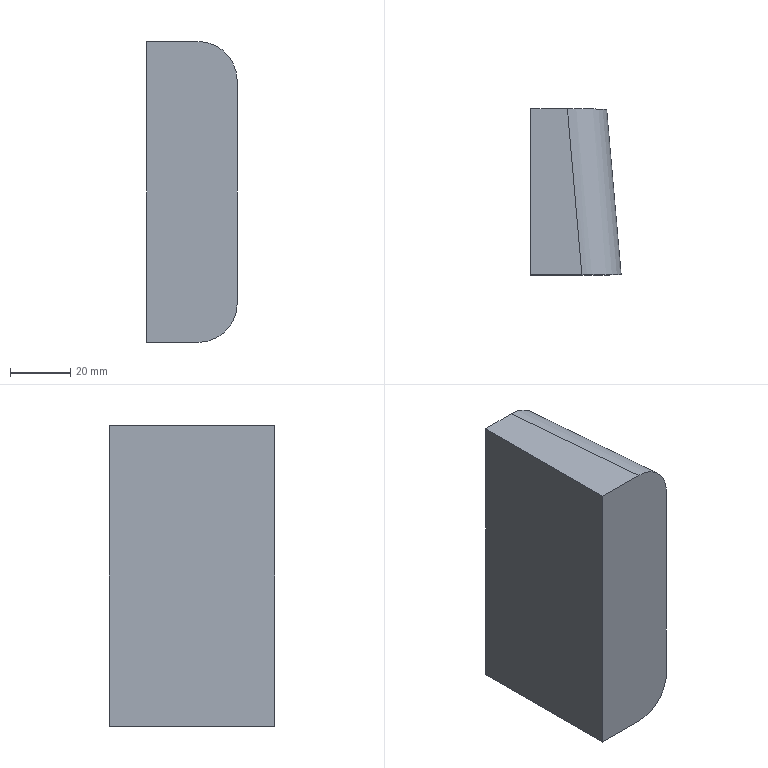Part | STEP file | 1 solid | 8 faces | box 30 x 55 x 100 mm | volume 147763 mm3 | plane 6 | cylinder 2 | commonest cylinder face diameters 26 x2
STEP:
#1=CARTESIAN_POINT('',(0.,0.,0.));
#2=DIRECTION('',(0.,0.,1.));
#3=DIRECTION('',(1.,0.,0.));
#4=AXIS2_PLACEMENT_3D('',#1,#2,#3);
#5=CARTESIAN_POINT('',(37.138,70.5,-11.47));
#6=VERTEX_POINT('',#5);
#7=CARTESIAN_POINT('',(54.088,70.5,-11.47));
#8=VERTEX_POINT('',#7);
#9=CARTESIAN_POINT('',(37.138,70.5,-11.47));
#10=DIRECTION('',(1.,0.,0.));
#11=VECTOR('',#10,1.);
#12=LINE('',#9,#11);
#13=CARTESIAN_POINT('',(-72.862,70.5,580.53));
#14=DIRECTION('',(0.,1.,0.));
#15=DIRECTION('',(0.,0.,1.));
#16=AXIS2_PLACEMENT_3D('',#13,#14,#15);
#17=PLANE('',#16);
#18=CARTESIAN_POINT('',(-592.,110.));
#19=DIRECTION('',(0.,1.));
#20=VECTOR('',#19,1.);
#21=LINE('',#18,#20);
#22=(GEOMETRIC_REPRESENTATION_CONTEXT(2)PARAMETRIC_REPRESENTATION_CONTEXT()REPRESENTATION_CONTEXT('',''));
#23=DEFINITIONAL_REPRESENTATION('',(#21),#22);
#24=PCURVE('',#17,#23);
#25=CARTESIAN_POINT('',(37.138,-9.5,-11.47));
#26=DIRECTION('',(0.,0.,1.));
#27=DIRECTION('',(-1.,0.,0.));
#28=AXIS2_PLACEMENT_3D('',#25,#26,#27);
#29=PLANE('',#28);
#30=CARTESIAN_POINT('',(0.,-80.));
#31=DIRECTION('',(-1.,0.));
#32=VECTOR('',#31,1.);
#33=LINE('',#30,#32);
#34=(GEOMETRIC_REPRESENTATION_CONTEXT(2)PARAMETRIC_REPRESENTATION_CONTEXT()REPRESENTATION_CONTEXT('',''));
#35=DEFINITIONAL_REPRESENTATION('',(#33),#34);
#36=PCURVE('',#29,#35);
#37=SURFACE_CURVE('',#12,(#24,#36),.PCURVE_S1.);
#38=EDGE_CURVE('',#6,#8,#37,.T.);
#39=ORIENTED_EDGE('',*,*,#38,.T.);
#40=CARTESIAN_POINT('',(67.138,70.5,1.53));
#41=VERTEX_POINT('',#40);
#42=CARTESIAN_POINT('',(54.088,70.5,-11.47));
#43=CARTESIAN_POINT('',(61.732,70.5,-11.47));
#44=CARTESIAN_POINT('',(67.138,70.5,-6.086));
#45=CARTESIAN_POINT('',(67.138,70.5,1.53));
#46=(BOUNDED_CURVE()B_SPLINE_CURVE(3,(#42,#43,#44,#45),.UNSPECIFIED.,.F.,.F.)B_SPLINE_CURVE_WITH_KNOTS((4,4),(1.571,3.142),.PIECEWISE_BEZIER_KNOTS.)CURVE()GEOMETRIC_REPRESENTATION_ITEM()RATIONAL_B_SPLINE_CURVE((1.,0.8047,0.8047,1.))REPRESENTATION_ITEM(''));
#47=CARTESIAN_POINT('',(-592.,126.95));
#48=CARTESIAN_POINT('',(-592.,134.595));
#49=CARTESIAN_POINT('',(-586.615,140.));
#50=CARTESIAN_POINT('',(-579.,140.));
#51=(BOUNDED_CURVE()B_SPLINE_CURVE(3,(#47,#48,#49,#50),.UNSPECIFIED.,.F.,.F.)B_SPLINE_CURVE_WITH_KNOTS((4,4),(1.571,3.142),.PIECEWISE_BEZIER_KNOTS.)CURVE()GEOMETRIC_REPRESENTATION_ITEM()RATIONAL_B_SPLINE_CURVE((1.,0.8047,0.8047,1.))REPRESENTATION_ITEM(''));
#52=(GEOMETRIC_REPRESENTATION_CONTEXT(2)PARAMETRIC_REPRESENTATION_CONTEXT()REPRESENTATION_CONTEXT('',''));
#53=DEFINITIONAL_REPRESENTATION('',(#51),#52);
#54=PCURVE('',#17,#53);
#55=CARTESIAN_POINT('',(54.187,69.367,1.53));
#56=DIRECTION('',(-0.08716,0.9962,0.));
#57=DIRECTION('',(0.9962,0.08716,0.));
#58=AXIS2_PLACEMENT_3D('',#55,#56,#57);
#59=CYLINDRICAL_SURFACE('',#58,13.);
#60=CARTESIAN_POINT('',(1.571,1.137));
#61=CARTESIAN_POINT('',(1.549,1.113));
#62=CARTESIAN_POINT('',(1.506,1.064));
#63=CARTESIAN_POINT('',(1.439,0.988));
#64=CARTESIAN_POINT('',(1.371,0.9113));
#65=CARTESIAN_POINT('',(1.301,0.834));
#66=CARTESIAN_POINT('',(1.23,0.7569));
#67=CARTESIAN_POINT('',(1.158,0.6804));
#68=CARTESIAN_POINT('',(1.085,0.6054));
#69=CARTESIAN_POINT('',(1.01,0.5323));
#70=CARTESIAN_POINT('',(0.9358,0.4621));
#71=CARTESIAN_POINT('',(0.8607,0.3952));
#72=CARTESIAN_POINT('',(0.7854,0.3324));
#73=CARTESIAN_POINT('',(0.7101,0.2741));
#74=CARTESIAN_POINT('',(0.635,0.2208));
#75=CARTESIAN_POINT('',(0.5603,0.173));
#76=CARTESIAN_POINT('',(0.4863,0.1309));
#77=CARTESIAN_POINT('',(0.413,0.09472));
#78=CARTESIAN_POINT('',(0.3408,0.06449));
#79=CARTESIAN_POINT('',(0.2697,0.04021));
#80=CARTESIAN_POINT('',(0.2,0.02178));
#81=CARTESIAN_POINT('',(0.1316,0.008981));
#82=CARTESIAN_POINT('',(0.06485,0.001569));
#83=CARTESIAN_POINT('',(0.02143,-0.000003694));
#84=CARTESIAN_POINT('',(0.,0.));
#85=B_SPLINE_CURVE_WITH_KNOTS('',3,(#60,#61,#62,#63,#64,#65,#66,#67,#68,#69,#70,#71,#72,#73,#74,#75,#76,#77,#78,#79,#80,#81,#82,#83,#84),.UNSPECIFIED.,.F.,.F.,(4,1,1,1,1,1,1,1,1,1,1,1,1,1,1,1,1,1,1,1,1,1,4),(1.571,1.642,1.714,1.785,1.856,1.928,1.999,2.071,2.142,2.213,2.285,2.356,2.428,2.499,2.57,2.642,2.713,2.785,2.856,2.927,2.999,3.07,3.142),.QUASI_UNIFORM_KNOTS.);
#86=(GEOMETRIC_REPRESENTATION_CONTEXT(2)PARAMETRIC_REPRESENTATION_CONTEXT()REPRESENTATION_CONTEXT('',''));
#87=DEFINITIONAL_REPRESENTATION('',(#85),#86);
#88=PCURVE('',#59,#87);
#89=SURFACE_CURVE('',#46,(#54,#88),.PCURVE_S1.);
#90=EDGE_CURVE('',#8,#41,#89,.T.);
#91=ORIENTED_EDGE('',*,*,#90,.T.);
#92=CARTESIAN_POINT('',(67.138,70.5,75.53));
#93=VERTEX_POINT('',#92);
#94=CARTESIAN_POINT('',(67.138,70.5,38.53));
#95=DIRECTION('',(0.,0.,1.));
#96=VECTOR('',#95,1.);
#97=LINE('',#94,#96);
#98=CARTESIAN_POINT('',(-542.,140.));
#99=DIRECTION('',(1.,0.));
#100=VECTOR('',#99,1.);
#101=LINE('',#98,#100);
#102=(GEOMETRIC_REPRESENTATION_CONTEXT(2)PARAMETRIC_REPRESENTATION_CONTEXT()REPRESENTATION_CONTEXT('',''));
#103=DEFINITIONAL_REPRESENTATION('',(#101),#102);
#104=PCURVE('',#17,#103);
#105=CARTESIAN_POINT('',(67.138,70.5,38.53));
#106=DIRECTION('',(-0.9962,-0.08716,0.));
#107=DIRECTION('',(-0.08716,0.9962,0.));
#108=AXIS2_PLACEMENT_3D('',#105,#106,#107);
#109=PLANE('',#108);
#110=CARTESIAN_POINT('',(0.,0.));
#111=DIRECTION('',(0.,-1.));
#112=VECTOR('',#111,1.);
#113=LINE('',#110,#112);
#114=(GEOMETRIC_REPRESENTATION_CONTEXT(2)PARAMETRIC_REPRESENTATION_CONTEXT()REPRESENTATION_CONTEXT('',''));
#115=DEFINITIONAL_REPRESENTATION('',(#113),#114);
#116=PCURVE('',#109,#115);
#117=SURFACE_CURVE('',#97,(#104,#116),.PCURVE_S1.);
#118=EDGE_CURVE('',#41,#93,#117,.T.);
#119=ORIENTED_EDGE('',*,*,#118,.T.);
#120=CARTESIAN_POINT('',(54.088,70.5,88.53));
#121=VERTEX_POINT('',#120);
#122=CARTESIAN_POINT('',(67.138,70.5,75.53));
#123=CARTESIAN_POINT('',(67.138,70.5,83.145));
#124=CARTESIAN_POINT('',(61.732,70.5,88.53));
#125=CARTESIAN_POINT('',(54.088,70.5,88.53));
#126=(BOUNDED_CURVE()B_SPLINE_CURVE(3,(#122,#123,#124,#125),.UNSPECIFIED.,.F.,.F.)B_SPLINE_CURVE_WITH_KNOTS((4,4),(3.142,4.712),.PIECEWISE_BEZIER_KNOTS.)CURVE()GEOMETRIC_REPRESENTATION_ITEM()RATIONAL_B_SPLINE_CURVE((1.,0.8047,0.8047,1.))REPRESENTATION_ITEM(''));
#127=CARTESIAN_POINT('',(-505.,140.));
#128=CARTESIAN_POINT('',(-497.385,140.));
#129=CARTESIAN_POINT('',(-492.,134.595));
#130=CARTESIAN_POINT('',(-492.,126.95));
#131=(BOUNDED_CURVE()B_SPLINE_CURVE(3,(#127,#128,#129,#130),.UNSPECIFIED.,.F.,.F.)B_SPLINE_CURVE_WITH_KNOTS((4,4),(3.142,4.712),.PIECEWISE_BEZIER_KNOTS.)CURVE()GEOMETRIC_REPRESENTATION_ITEM()RATIONAL_B_SPLINE_CURVE((1.,0.8047,0.8047,1.))REPRESENTATION_ITEM(''));
#132=(GEOMETRIC_REPRESENTATION_CONTEXT(2)PARAMETRIC_REPRESENTATION_CONTEXT()REPRESENTATION_CONTEXT('',''));
#133=DEFINITIONAL_REPRESENTATION('',(#131),#132);
#134=PCURVE('',#17,#133);
#135=CARTESIAN_POINT('',(61.057,-9.157,75.53));
#136=DIRECTION('',(-0.08716,0.9962,0.));
#137=DIRECTION('',(0.9962,0.08716,0.));
#138=AXIS2_PLACEMENT_3D('',#135,#136,#137);
#139=CYLINDRICAL_SURFACE('',#138,13.);
#140=CARTESIAN_POINT('',(6.283,78.824));
#141=CARTESIAN_POINT('',(6.262,78.824));
#142=CARTESIAN_POINT('',(6.218,78.826));
#143=CARTESIAN_POINT('',(6.152,78.833));
#144=CARTESIAN_POINT('',(6.083,78.846));
#145=CARTESIAN_POINT('',(6.013,78.864));
#146=CARTESIAN_POINT('',(5.942,78.889));
#147=CARTESIAN_POINT('',(5.87,78.919));
#148=CARTESIAN_POINT('',(5.797,78.955));
#149=CARTESIAN_POINT('',(5.723,78.997));
#150=CARTESIAN_POINT('',(5.648,79.045));
#151=CARTESIAN_POINT('',(5.573,79.098));
#152=CARTESIAN_POINT('',(5.498,79.156));
#153=CARTESIAN_POINT('',(5.422,79.219));
#154=CARTESIAN_POINT('',(5.347,79.286));
#155=CARTESIAN_POINT('',(5.273,79.356));
#156=CARTESIAN_POINT('',(5.199,79.429));
#157=CARTESIAN_POINT('',(5.125,79.504));
#158=CARTESIAN_POINT('',(5.053,79.581));
#159=CARTESIAN_POINT('',(4.982,79.658));
#160=CARTESIAN_POINT('',(4.912,79.735));
#161=CARTESIAN_POINT('',(4.844,79.812));
#162=CARTESIAN_POINT('',(4.777,79.888));
#163=CARTESIAN_POINT('',(4.734,79.937));
#164=CARTESIAN_POINT('',(4.712,79.961));
#165=B_SPLINE_CURVE_WITH_KNOTS('',3,(#140,#141,#142,#143,#144,#145,#146,#147,#148,#149,#150,#151,#152,#153,#154,#155,#156,#157,#158,#159,#160,#161,#162,#163,#164),.UNSPECIFIED.,.F.,.F.,(4,1,1,1,1,1,1,1,1,1,1,1,1,1,1,1,1,1,1,1,1,1,4),(3.142,3.213,3.284,3.356,3.427,3.499,3.57,3.641,3.713,3.784,3.856,3.927,3.998,4.07,4.141,4.213,4.284,4.355,4.427,4.498,4.57,4.641,4.712),.QUASI_UNIFORM_KNOTS.);
#166=(GEOMETRIC_REPRESENTATION_CONTEXT(2)PARAMETRIC_REPRESENTATION_CONTEXT()REPRESENTATION_CONTEXT('',''));
#167=DEFINITIONAL_REPRESENTATION('',(#165),#166);
#168=PCURVE('',#139,#167);
#169=SURFACE_CURVE('',#126,(#134,#168),.PCURVE_S1.);
#170=EDGE_CURVE('',#93,#121,#169,.T.);
#171=ORIENTED_EDGE('',*,*,#170,.T.);
#172=CARTESIAN_POINT('',(37.138,70.5,88.53));
#173=VERTEX_POINT('',#172);
#174=CARTESIAN_POINT('',(57.138,70.5,88.53));
#175=DIRECTION('',(-1.,0.,0.));
#176=VECTOR('',#175,1.);
#177=LINE('',#174,#176);
#178=CARTESIAN_POINT('',(-492.,130.));
#179=DIRECTION('',(0.,-1.));
#180=VECTOR('',#179,1.);
#181=LINE('',#178,#180);
#182=(GEOMETRIC_REPRESENTATION_CONTEXT(2)PARAMETRIC_REPRESENTATION_CONTEXT()REPRESENTATION_CONTEXT('',''));
#183=DEFINITIONAL_REPRESENTATION('',(#181),#182);
#184=PCURVE('',#17,#183);
#185=CARTESIAN_POINT('',(57.138,-9.5,88.53));
#186=DIRECTION('',(0.,0.,-1.));
#187=DIRECTION('',(1.,0.,0.));
#188=AXIS2_PLACEMENT_3D('',#185,#186,#187);
#189=PLANE('',#188);
#190=CARTESIAN_POINT('',(0.,-80.));
#191=DIRECTION('',(-1.,0.));
#192=VECTOR('',#191,1.);
#193=LINE('',#190,#192);
#194=(GEOMETRIC_REPRESENTATION_CONTEXT(2)PARAMETRIC_REPRESENTATION_CONTEXT()REPRESENTATION_CONTEXT('',''));
#195=DEFINITIONAL_REPRESENTATION('',(#193),#194);
#196=PCURVE('',#189,#195);
#197=SURFACE_CURVE('',#177,(#184,#196),.PCURVE_S1.);
#198=EDGE_CURVE('',#121,#173,#197,.T.);
#199=ORIENTED_EDGE('',*,*,#198,.T.);
#200=CARTESIAN_POINT('',(37.138,70.5,88.53));
#201=DIRECTION('',(0.,0.,-1.));
#202=VECTOR('',#201,1.);
#203=LINE('',#200,#202);
#204=CARTESIAN_POINT('',(-492.,110.));
#205=DIRECTION('',(-1.,0.));
#206=VECTOR('',#205,1.);
#207=LINE('',#204,#206);
#208=(GEOMETRIC_REPRESENTATION_CONTEXT(2)PARAMETRIC_REPRESENTATION_CONTEXT()REPRESENTATION_CONTEXT('',''));
#209=DEFINITIONAL_REPRESENTATION('',(#207),#208);
#210=PCURVE('',#17,#209);
#211=CARTESIAN_POINT('',(37.138,-9.5,88.53));
#212=DIRECTION('',(1.,0.,0.));
#213=DIRECTION('',(0.,0.,1.));
#214=AXIS2_PLACEMENT_3D('',#211,#212,#213);
#215=PLANE('',#214);
#216=CARTESIAN_POINT('',(0.,-80.));
#217=DIRECTION('',(-1.,0.));
#218=VECTOR('',#217,1.);
#219=LINE('',#216,#218);
#220=(GEOMETRIC_REPRESENTATION_CONTEXT(2)PARAMETRIC_REPRESENTATION_CONTEXT()REPRESENTATION_CONTEXT('',''));
#221=DEFINITIONAL_REPRESENTATION('',(#219),#220);
#222=PCURVE('',#215,#221);
#223=SURFACE_CURVE('',#203,(#210,#222),.PCURVE_S1.);
#224=EDGE_CURVE('',#173,#6,#223,.T.);
#225=ORIENTED_EDGE('',*,*,#224,.T.);
#226=EDGE_LOOP('',(#39,#91,#119,#171,#199,#225));
#227=FACE_BOUND('',#226,.T.);
#228=ADVANCED_FACE('',(#227),#17,.F.);
#229=CARTESIAN_POINT('',(49.276,125.5,88.53));
#230=VERTEX_POINT('',#229);
#231=CARTESIAN_POINT('',(61.057,-9.157,88.53));
#232=DIRECTION('',(-0.08716,0.9962,0.));
#233=VECTOR('',#232,1.);
#234=LINE('',#231,#233);
#235=CARTESIAN_POINT('',(3.919,-0.3429));
#236=DIRECTION('',(-0.08716,-0.9962));
#237=VECTOR('',#236,1.);
#238=LINE('',#235,#237);
#239=(GEOMETRIC_REPRESENTATION_CONTEXT(2)PARAMETRIC_REPRESENTATION_CONTEXT()REPRESENTATION_CONTEXT('',''));
#240=DEFINITIONAL_REPRESENTATION('',(#238),#239);
#241=PCURVE('',#189,#240);
#242=CARTESIAN_POINT('',(4.712,0.));
#243=DIRECTION('',(0.,1.));
#244=VECTOR('',#243,1.);
#245=LINE('',#242,#244);
#246=(GEOMETRIC_REPRESENTATION_CONTEXT(2)PARAMETRIC_REPRESENTATION_CONTEXT()REPRESENTATION_CONTEXT('',''));
#247=DEFINITIONAL_REPRESENTATION('',(#245),#246);
#248=PCURVE('',#139,#247);
#249=SURFACE_CURVE('',#234,(#241,#248),.PCURVE_S1.);
#250=EDGE_CURVE('',#121,#230,#249,.T.);
#251=ORIENTED_EDGE('',*,*,#250,.T.);
#252=CARTESIAN_POINT('',(37.138,125.5,88.53));
#253=VERTEX_POINT('',#252);
#254=CARTESIAN_POINT('',(57.138,125.5,88.53));
#255=DIRECTION('',(-1.,0.,0.));
#256=VECTOR('',#255,1.);
#257=LINE('',#254,#256);
#258=CARTESIAN_POINT('',(0.,-135.));
#259=DIRECTION('',(-1.,0.));
#260=VECTOR('',#259,1.);
#261=LINE('',#258,#260);
#262=(GEOMETRIC_REPRESENTATION_CONTEXT(2)PARAMETRIC_REPRESENTATION_CONTEXT()REPRESENTATION_CONTEXT('',''));
#263=DEFINITIONAL_REPRESENTATION('',(#261),#262);
#264=PCURVE('',#189,#263);
#265=CARTESIAN_POINT('',(-72.362,125.5,-51.47));
#266=DIRECTION('',(0.,-1.,0.));
#267=DIRECTION('',(0.,0.,-1.));
#268=AXIS2_PLACEMENT_3D('',#265,#266,#267);
#269=PLANE('',#268);
#270=CARTESIAN_POINT('',(-140.,129.5));
#271=DIRECTION('',(0.,-1.));
#272=VECTOR('',#271,1.);
#273=LINE('',#270,#272);
#274=(GEOMETRIC_REPRESENTATION_CONTEXT(2)PARAMETRIC_REPRESENTATION_CONTEXT()REPRESENTATION_CONTEXT('',''));
#275=DEFINITIONAL_REPRESENTATION('',(#273),#274);
#276=PCURVE('',#269,#275);
#277=SURFACE_CURVE('',#257,(#264,#276),.PCURVE_S1.);
#278=EDGE_CURVE('',#230,#253,#277,.T.);
#279=ORIENTED_EDGE('',*,*,#278,.T.);
#280=CARTESIAN_POINT('',(37.138,-9.5,88.53));
#281=DIRECTION('',(0.,1.,0.));
#282=VECTOR('',#281,1.);
#283=LINE('',#280,#282);
#284=CARTESIAN_POINT('',(-20.,0.));
#285=DIRECTION('',(0.,-1.));
#286=VECTOR('',#285,1.);
#287=LINE('',#284,#286);
#288=(GEOMETRIC_REPRESENTATION_CONTEXT(2)PARAMETRIC_REPRESENTATION_CONTEXT()REPRESENTATION_CONTEXT('',''));
#289=DEFINITIONAL_REPRESENTATION('',(#287),#288);
#290=PCURVE('',#189,#289);
#291=CARTESIAN_POINT('',(0.,0.));
#292=DIRECTION('',(0.,-1.));
#293=VECTOR('',#292,1.);
#294=LINE('',#291,#293);
#295=(GEOMETRIC_REPRESENTATION_CONTEXT(2)PARAMETRIC_REPRESENTATION_CONTEXT()REPRESENTATION_CONTEXT('',''));
#296=DEFINITIONAL_REPRESENTATION('',(#294),#295);
#297=PCURVE('',#215,#296);
#298=SURFACE_CURVE('',#283,(#290,#297),.PCURVE_S1.);
#299=EDGE_CURVE('',#173,#253,#298,.T.);
#300=ORIENTED_EDGE('',*,*,#299,.F.);
#301=ORIENTED_EDGE('',*,*,#198,.F.);
#302=EDGE_LOOP('',(#251,#279,#300,#301));
#303=FACE_BOUND('',#302,.T.);
#304=ADVANCED_FACE('',(#303),#189,.F.);
#305=CARTESIAN_POINT('',(62.326,125.5,1.53));
#306=VERTEX_POINT('',#305);
#307=CARTESIAN_POINT('',(67.138,70.5,1.53));
#308=DIRECTION('',(-0.08716,0.9962,0.));
#309=VECTOR('',#308,1.);
#310=LINE('',#307,#309);
#311=CARTESIAN_POINT('',(0.,37.));
#312=DIRECTION('',(1.,0.));
#313=VECTOR('',#312,1.);
#314=LINE('',#311,#313);
#315=(GEOMETRIC_REPRESENTATION_CONTEXT(2)PARAMETRIC_REPRESENTATION_CONTEXT()REPRESENTATION_CONTEXT('',''));
#316=DEFINITIONAL_REPRESENTATION('',(#314),#315);
#317=PCURVE('',#109,#316);
#318=CARTESIAN_POINT('',(0.,0.));
#319=DIRECTION('',(0.,1.));
#320=VECTOR('',#319,1.);
#321=LINE('',#318,#320);
#322=(GEOMETRIC_REPRESENTATION_CONTEXT(2)PARAMETRIC_REPRESENTATION_CONTEXT()REPRESENTATION_CONTEXT('',''));
#323=DEFINITIONAL_REPRESENTATION('',(#321),#322);
#324=PCURVE('',#59,#323);
#325=SURFACE_CURVE('',#310,(#317,#324),.PCURVE_S1.);
#326=EDGE_CURVE('',#41,#306,#325,.T.);
#327=ORIENTED_EDGE('',*,*,#326,.T.);
#328=CARTESIAN_POINT('',(62.326,125.5,75.53));
#329=VERTEX_POINT('',#328);
#330=CARTESIAN_POINT('',(62.326,125.5,38.53));
#331=DIRECTION('',(0.,0.,1.));
#332=VECTOR('',#331,1.);
#333=LINE('',#330,#332);
#334=CARTESIAN_POINT('',(55.21,0.));
#335=DIRECTION('',(0.,-1.));
#336=VECTOR('',#335,1.);
#337=LINE('',#334,#336);
#338=(GEOMETRIC_REPRESENTATION_CONTEXT(2)PARAMETRIC_REPRESENTATION_CONTEXT()REPRESENTATION_CONTEXT('',''));
#339=DEFINITIONAL_REPRESENTATION('',(#337),#338);
#340=PCURVE('',#109,#339);
#341=CARTESIAN_POINT('',(-90.,134.688));
#342=DIRECTION('',(-1.,0.));
#343=VECTOR('',#342,1.);
#344=LINE('',#341,#343);
#345=(GEOMETRIC_REPRESENTATION_CONTEXT(2)PARAMETRIC_REPRESENTATION_CONTEXT()REPRESENTATION_CONTEXT('',''));
#346=DEFINITIONAL_REPRESENTATION('',(#344),#345);
#347=PCURVE('',#269,#346);
#348=SURFACE_CURVE('',#333,(#340,#347),.PCURVE_S1.);
#349=EDGE_CURVE('',#306,#329,#348,.T.);
#350=ORIENTED_EDGE('',*,*,#349,.T.);
#351=CARTESIAN_POINT('',(67.138,70.5,75.53));
#352=DIRECTION('',(0.08716,-0.9962,0.));
#353=VECTOR('',#352,1.);
#354=LINE('',#351,#353);
#355=CARTESIAN_POINT('',(0.,-37.));
#356=DIRECTION('',(-1.,0.));
#357=VECTOR('',#356,1.);
#358=LINE('',#355,#357);
#359=(GEOMETRIC_REPRESENTATION_CONTEXT(2)PARAMETRIC_REPRESENTATION_CONTEXT()REPRESENTATION_CONTEXT('',''));
#360=DEFINITIONAL_REPRESENTATION('',(#358),#359);
#361=PCURVE('',#109,#360);
#362=CARTESIAN_POINT('',(6.283,78.824));
#363=DIRECTION('',(0.,-1.));
#364=VECTOR('',#363,1.);
#365=LINE('',#362,#364);
#366=(GEOMETRIC_REPRESENTATION_CONTEXT(2)PARAMETRIC_REPRESENTATION_CONTEXT()REPRESENTATION_CONTEXT('',''));
#367=DEFINITIONAL_REPRESENTATION('',(#365),#366);
#368=PCURVE('',#139,#367);
#369=SURFACE_CURVE('',#354,(#361,#368),.PCURVE_S1.);
#370=EDGE_CURVE('',#329,#93,#369,.T.);
#371=ORIENTED_EDGE('',*,*,#370,.T.);
#372=ORIENTED_EDGE('',*,*,#118,.F.);
#373=EDGE_LOOP('',(#327,#350,#371,#372));
#374=FACE_BOUND('',#373,.T.);
#375=ADVANCED_FACE('',(#374),#109,.F.);
#376=CARTESIAN_POINT('',(37.138,125.5,-11.47));
#377=VERTEX_POINT('',#376);
#378=CARTESIAN_POINT('',(37.138,-9.5,-11.47));
#379=DIRECTION('',(0.,1.,0.));
#380=VECTOR('',#379,1.);
#381=LINE('',#378,#380);
#382=CARTESIAN_POINT('',(0.,0.));
#383=DIRECTION('',(0.,-1.));
#384=VECTOR('',#383,1.);
#385=LINE('',#382,#384);
#386=(GEOMETRIC_REPRESENTATION_CONTEXT(2)PARAMETRIC_REPRESENTATION_CONTEXT()REPRESENTATION_CONTEXT('',''));
#387=DEFINITIONAL_REPRESENTATION('',(#385),#386);
#388=PCURVE('',#29,#387);
#389=CARTESIAN_POINT('',(-100.,0.));
#390=DIRECTION('',(0.,-1.));
#391=VECTOR('',#390,1.);
#392=LINE('',#389,#391);
#393=(GEOMETRIC_REPRESENTATION_CONTEXT(2)PARAMETRIC_REPRESENTATION_CONTEXT()REPRESENTATION_CONTEXT('',''));
#394=DEFINITIONAL_REPRESENTATION('',(#392),#393);
#395=PCURVE('',#215,#394);
#396=SURFACE_CURVE('',#381,(#388,#395),.PCURVE_S1.);
#397=EDGE_CURVE('',#6,#377,#396,.T.);
#398=ORIENTED_EDGE('',*,*,#397,.T.);
#399=CARTESIAN_POINT('',(49.276,125.5,-11.47));
#400=VERTEX_POINT('',#399);
#401=CARTESIAN_POINT('',(37.138,125.5,-11.47));
#402=DIRECTION('',(1.,0.,0.));
#403=VECTOR('',#402,1.);
#404=LINE('',#401,#403);
#405=CARTESIAN_POINT('',(0.,-135.));
#406=DIRECTION('',(-1.,0.));
#407=VECTOR('',#406,1.);
#408=LINE('',#405,#407);
#409=(GEOMETRIC_REPRESENTATION_CONTEXT(2)PARAMETRIC_REPRESENTATION_CONTEXT()REPRESENTATION_CONTEXT('',''));
#410=DEFINITIONAL_REPRESENTATION('',(#408),#409);
#411=PCURVE('',#29,#410);
#412=CARTESIAN_POINT('',(-40.,109.5));
#413=DIRECTION('',(0.,1.));
#414=VECTOR('',#413,1.);
#415=LINE('',#412,#414);
#416=(GEOMETRIC_REPRESENTATION_CONTEXT(2)PARAMETRIC_REPRESENTATION_CONTEXT()REPRESENTATION_CONTEXT('',''));
#417=DEFINITIONAL_REPRESENTATION('',(#415),#416);
#418=PCURVE('',#269,#417);
#419=SURFACE_CURVE('',#404,(#411,#418),.PCURVE_S1.);
#420=EDGE_CURVE('',#377,#400,#419,.T.);
#421=ORIENTED_EDGE('',*,*,#420,.T.);
#422=CARTESIAN_POINT('',(60.905,-7.421,-11.47));
#423=DIRECTION('',(0.08716,-0.9962,0.));
#424=VECTOR('',#423,1.);
#425=LINE('',#422,#424);
#426=CARTESIAN_POINT('',(-23.768,-2.079));
#427=DIRECTION('',(-0.08716,0.9962));
#428=VECTOR('',#427,1.);
#429=LINE('',#426,#428);
#430=(GEOMETRIC_REPRESENTATION_CONTEXT(2)PARAMETRIC_REPRESENTATION_CONTEXT()REPRESENTATION_CONTEXT('',''));
#431=DEFINITIONAL_REPRESENTATION('',(#429),#430);
#432=PCURVE('',#29,#431);
#433=CARTESIAN_POINT('',(1.571,-77.081));
#434=DIRECTION('',(0.,-1.));
#435=VECTOR('',#434,1.);
#436=LINE('',#433,#435);
#437=(GEOMETRIC_REPRESENTATION_CONTEXT(2)PARAMETRIC_REPRESENTATION_CONTEXT()REPRESENTATION_CONTEXT('',''));
#438=DEFINITIONAL_REPRESENTATION('',(#436),#437);
#439=PCURVE('',#59,#438);
#440=SURFACE_CURVE('',#425,(#432,#439),.PCURVE_S1.);
#441=EDGE_CURVE('',#400,#8,#440,.T.);
#442=ORIENTED_EDGE('',*,*,#441,.T.);
#443=ORIENTED_EDGE('',*,*,#38,.F.);
#444=EDGE_LOOP('',(#398,#421,#442,#443));
#445=FACE_BOUND('',#444,.T.);
#446=ADVANCED_FACE('',(#445),#29,.F.);
#447=ORIENTED_EDGE('',*,*,#299,.T.);
#448=CARTESIAN_POINT('',(37.138,125.5,88.53));
#449=DIRECTION('',(0.,0.,-1.));
#450=VECTOR('',#449,1.);
#451=LINE('',#448,#450);
#452=CARTESIAN_POINT('',(0.,-135.));
#453=DIRECTION('',(-1.,0.));
#454=VECTOR('',#453,1.);
#455=LINE('',#452,#454);
#456=(GEOMETRIC_REPRESENTATION_CONTEXT(2)PARAMETRIC_REPRESENTATION_CONTEXT()REPRESENTATION_CONTEXT('',''));
#457=DEFINITIONAL_REPRESENTATION('',(#455),#456);
#458=PCURVE('',#215,#457);
#459=CARTESIAN_POINT('',(-140.,109.5));
#460=DIRECTION('',(1.,0.));
#461=VECTOR('',#460,1.);
#462=LINE('',#459,#461);
#463=(GEOMETRIC_REPRESENTATION_CONTEXT(2)PARAMETRIC_REPRESENTATION_CONTEXT()REPRESENTATION_CONTEXT('',''));
#464=DEFINITIONAL_REPRESENTATION('',(#462),#463);
#465=PCURVE('',#269,#464);
#466=SURFACE_CURVE('',#451,(#458,#465),.PCURVE_S1.);
#467=EDGE_CURVE('',#253,#377,#466,.T.);
#468=ORIENTED_EDGE('',*,*,#467,.T.);
#469=ORIENTED_EDGE('',*,*,#397,.F.);
#470=ORIENTED_EDGE('',*,*,#224,.F.);
#471=EDGE_LOOP('',(#447,#468,#469,#470));
#472=FACE_BOUND('',#471,.T.);
#473=ADVANCED_FACE('',(#472),#215,.F.);
#474=CARTESIAN_POINT('',(62.326,125.5,1.53));
#475=CARTESIAN_POINT('',(62.326,125.5,-6.086));
#476=CARTESIAN_POINT('',(56.92,125.5,-11.47));
#477=CARTESIAN_POINT('',(49.276,125.5,-11.47));
#478=(BOUNDED_CURVE()B_SPLINE_CURVE(3,(#474,#475,#476,#477),.UNSPECIFIED.,.F.,.F.)B_SPLINE_CURVE_WITH_KNOTS((4,4),(3.142,4.712),.PIECEWISE_BEZIER_KNOTS.)CURVE()GEOMETRIC_REPRESENTATION_ITEM()RATIONAL_B_SPLINE_CURVE((1.,0.8047,0.8047,1.))REPRESENTATION_ITEM(''));
#479=CARTESIAN_POINT('',(0.,55.21));
#480=CARTESIAN_POINT('',(0.02143,55.21));
#481=CARTESIAN_POINT('',(0.06485,55.212));
#482=CARTESIAN_POINT('',(0.1316,55.219));
#483=CARTESIAN_POINT('',(0.2,55.232));
#484=CARTESIAN_POINT('',(0.2697,55.25));
#485=CARTESIAN_POINT('',(0.3408,55.275));
#486=CARTESIAN_POINT('',(0.413,55.305));
#487=CARTESIAN_POINT('',(0.4863,55.341));
#488=CARTESIAN_POINT('',(0.5603,55.383));
#489=CARTESIAN_POINT('',(0.635,55.431));
#490=CARTESIAN_POINT('',(0.7101,55.484));
#491=CARTESIAN_POINT('',(0.7854,55.542));
#492=CARTESIAN_POINT('',(0.8607,55.605));
#493=CARTESIAN_POINT('',(0.9358,55.672));
#494=CARTESIAN_POINT('',(1.01,55.742));
#495=CARTESIAN_POINT('',(1.085,55.815));
#496=CARTESIAN_POINT('',(1.158,55.891));
#497=CARTESIAN_POINT('',(1.23,55.967));
#498=CARTESIAN_POINT('',(1.301,56.044));
#499=CARTESIAN_POINT('',(1.371,56.121));
#500=CARTESIAN_POINT('',(1.439,56.198));
#501=CARTESIAN_POINT('',(1.506,56.274));
#502=CARTESIAN_POINT('',(1.549,56.323));
#503=CARTESIAN_POINT('',(1.571,56.347));
#504=B_SPLINE_CURVE_WITH_KNOTS('',3,(#479,#480,#481,#482,#483,#484,#485,#486,#487,#488,#489,#490,#491,#492,#493,#494,#495,#496,#497,#498,#499,#500,#501,#502,#503),.UNSPECIFIED.,.F.,.F.,(4,1,1,1,1,1,1,1,1,1,1,1,1,1,1,1,1,1,1,1,1,1,4),(3.142,3.213,3.284,3.356,3.427,3.499,3.57,3.641,3.713,3.784,3.856,3.927,3.998,4.07,4.141,4.213,4.284,4.355,4.427,4.498,4.57,4.641,4.712),.QUASI_UNIFORM_KNOTS.);
#505=(GEOMETRIC_REPRESENTATION_CONTEXT(2)PARAMETRIC_REPRESENTATION_CONTEXT()REPRESENTATION_CONTEXT('',''));
#506=DEFINITIONAL_REPRESENTATION('',(#504),#505);
#507=PCURVE('',#59,#506);
#508=CARTESIAN_POINT('',(-53.,134.688));
#509=CARTESIAN_POINT('',(-45.385,134.688));
#510=CARTESIAN_POINT('',(-40.,129.283));
#511=CARTESIAN_POINT('',(-40.,121.638));
#512=(BOUNDED_CURVE()B_SPLINE_CURVE(3,(#508,#509,#510,#511),.UNSPECIFIED.,.F.,.F.)B_SPLINE_CURVE_WITH_KNOTS((4,4),(3.142,4.712),.PIECEWISE_BEZIER_KNOTS.)CURVE()GEOMETRIC_REPRESENTATION_ITEM()RATIONAL_B_SPLINE_CURVE((1.,0.8047,0.8047,1.))REPRESENTATION_ITEM(''));
#513=(GEOMETRIC_REPRESENTATION_CONTEXT(2)PARAMETRIC_REPRESENTATION_CONTEXT()REPRESENTATION_CONTEXT('',''));
#514=DEFINITIONAL_REPRESENTATION('',(#512),#513);
#515=PCURVE('',#269,#514);
#516=SURFACE_CURVE('',#478,(#507,#515),.PCURVE_S1.);
#517=EDGE_CURVE('',#306,#400,#516,.T.);
#518=ORIENTED_EDGE('',*,*,#517,.F.);
#519=ORIENTED_EDGE('',*,*,#326,.F.);
#520=ORIENTED_EDGE('',*,*,#90,.F.);
#521=ORIENTED_EDGE('',*,*,#441,.F.);
#522=EDGE_LOOP('',(#518,#519,#520,#521));
#523=FACE_BOUND('',#522,.T.);
#524=ADVANCED_FACE('',(#523),#59,.T.);
#525=CARTESIAN_POINT('',(49.276,125.5,88.53));
#526=CARTESIAN_POINT('',(56.92,125.5,88.53));
#527=CARTESIAN_POINT('',(62.326,125.5,83.145));
#528=CARTESIAN_POINT('',(62.326,125.5,75.53));
#529=(BOUNDED_CURVE()B_SPLINE_CURVE(3,(#525,#526,#527,#528),.UNSPECIFIED.,.F.,.F.)B_SPLINE_CURVE_WITH_KNOTS((4,4),(1.571,3.142),.PIECEWISE_BEZIER_KNOTS.)CURVE()GEOMETRIC_REPRESENTATION_ITEM()RATIONAL_B_SPLINE_CURVE((1.,0.8047,0.8047,1.))REPRESENTATION_ITEM(''));
#530=CARTESIAN_POINT('',(4.712,135.171));
#531=CARTESIAN_POINT('',(4.734,135.147));
#532=CARTESIAN_POINT('',(4.777,135.098));
#533=CARTESIAN_POINT('',(4.844,135.022));
#534=CARTESIAN_POINT('',(4.912,134.945));
#535=CARTESIAN_POINT('',(4.982,134.868));
#536=CARTESIAN_POINT('',(5.053,134.791));
#537=CARTESIAN_POINT('',(5.125,134.715));
#538=CARTESIAN_POINT('',(5.199,134.639));
#539=CARTESIAN_POINT('',(5.273,134.566));
#540=CARTESIAN_POINT('',(5.347,134.496));
#541=CARTESIAN_POINT('',(5.422,134.429));
#542=CARTESIAN_POINT('',(5.498,134.366));
#543=CARTESIAN_POINT('',(5.573,134.308));
#544=CARTESIAN_POINT('',(5.648,134.255));
#545=CARTESIAN_POINT('',(5.723,134.207));
#546=CARTESIAN_POINT('',(5.797,134.165));
#547=CARTESIAN_POINT('',(5.87,134.129));
#548=CARTESIAN_POINT('',(5.942,134.099));
#549=CARTESIAN_POINT('',(6.013,134.074));
#550=CARTESIAN_POINT('',(6.083,134.056));
#551=CARTESIAN_POINT('',(6.152,134.043));
#552=CARTESIAN_POINT('',(6.218,134.036));
#553=CARTESIAN_POINT('',(6.262,134.034));
#554=CARTESIAN_POINT('',(6.283,134.034));
#555=B_SPLINE_CURVE_WITH_KNOTS('',3,(#530,#531,#532,#533,#534,#535,#536,#537,#538,#539,#540,#541,#542,#543,#544,#545,#546,#547,#548,#549,#550,#551,#552,#553,#554),.UNSPECIFIED.,.F.,.F.,(4,1,1,1,1,1,1,1,1,1,1,1,1,1,1,1,1,1,1,1,1,1,4),(1.571,1.642,1.714,1.785,1.856,1.928,1.999,2.071,2.142,2.213,2.285,2.356,2.428,2.499,2.57,2.642,2.713,2.785,2.856,2.927,2.999,3.07,3.142),.QUASI_UNIFORM_KNOTS.);
#556=(GEOMETRIC_REPRESENTATION_CONTEXT(2)PARAMETRIC_REPRESENTATION_CONTEXT()REPRESENTATION_CONTEXT('',''));
#557=DEFINITIONAL_REPRESENTATION('',(#555),#556);
#558=PCURVE('',#139,#557);
#559=CARTESIAN_POINT('',(-140.,121.638));
#560=CARTESIAN_POINT('',(-140.,129.283));
#561=CARTESIAN_POINT('',(-134.615,134.688));
#562=CARTESIAN_POINT('',(-127.,134.688));
#563=(BOUNDED_CURVE()B_SPLINE_CURVE(3,(#559,#560,#561,#562),.UNSPECIFIED.,.F.,.F.)B_SPLINE_CURVE_WITH_KNOTS((4,4),(1.571,3.142),.PIECEWISE_BEZIER_KNOTS.)CURVE()GEOMETRIC_REPRESENTATION_ITEM()RATIONAL_B_SPLINE_CURVE((1.,0.8047,0.8047,1.))REPRESENTATION_ITEM(''));
#564=(GEOMETRIC_REPRESENTATION_CONTEXT(2)PARAMETRIC_REPRESENTATION_CONTEXT()REPRESENTATION_CONTEXT('',''));
#565=DEFINITIONAL_REPRESENTATION('',(#563),#564);
#566=PCURVE('',#269,#565);
#567=SURFACE_CURVE('',#529,(#558,#566),.PCURVE_S1.);
#568=EDGE_CURVE('',#230,#329,#567,.T.);
#569=ORIENTED_EDGE('',*,*,#568,.F.);
#570=ORIENTED_EDGE('',*,*,#250,.F.);
#571=ORIENTED_EDGE('',*,*,#170,.F.);
#572=ORIENTED_EDGE('',*,*,#370,.F.);
#573=EDGE_LOOP('',(#569,#570,#571,#572));
#574=FACE_BOUND('',#573,.T.);
#575=ADVANCED_FACE('',(#574),#139,.T.);
#576=ORIENTED_EDGE('',*,*,#467,.F.);
#577=ORIENTED_EDGE('',*,*,#278,.F.);
#578=ORIENTED_EDGE('',*,*,#568,.T.);
#579=ORIENTED_EDGE('',*,*,#349,.F.);
#580=ORIENTED_EDGE('',*,*,#517,.T.);
#581=ORIENTED_EDGE('',*,*,#420,.F.);
#582=EDGE_LOOP('',(#576,#577,#578,#579,#580,#581));
#583=FACE_BOUND('',#582,.T.);
#584=ADVANCED_FACE('',(#583),#269,.F.);
#585=CLOSED_SHELL('',(#228,#304,#375,#446,#473,#524,#575,#584));
#586=MANIFOLD_SOLID_BREP('',#585);
#587=(LENGTH_UNIT()NAMED_UNIT(*)SI_UNIT(.MILLI.,.METRE.));
#588=UNCERTAINTY_MEASURE_WITH_UNIT(LENGTH_MEASURE(0.0000001),#587,'','');
#589=(NAMED_UNIT(*)PLANE_ANGLE_UNIT()SI_UNIT($,.RADIAN.));
#590=(NAMED_UNIT(*)SI_UNIT($,.STERADIAN.)SOLID_ANGLE_UNIT());
#591=(GEOMETRIC_REPRESENTATION_CONTEXT(3)GLOBAL_UNCERTAINTY_ASSIGNED_CONTEXT((#588))GLOBAL_UNIT_ASSIGNED_CONTEXT((#587,#589,#590))REPRESENTATION_CONTEXT('',''));
#592=ADVANCED_BREP_SHAPE_REPRESENTATION('',(#4,#586),#591);